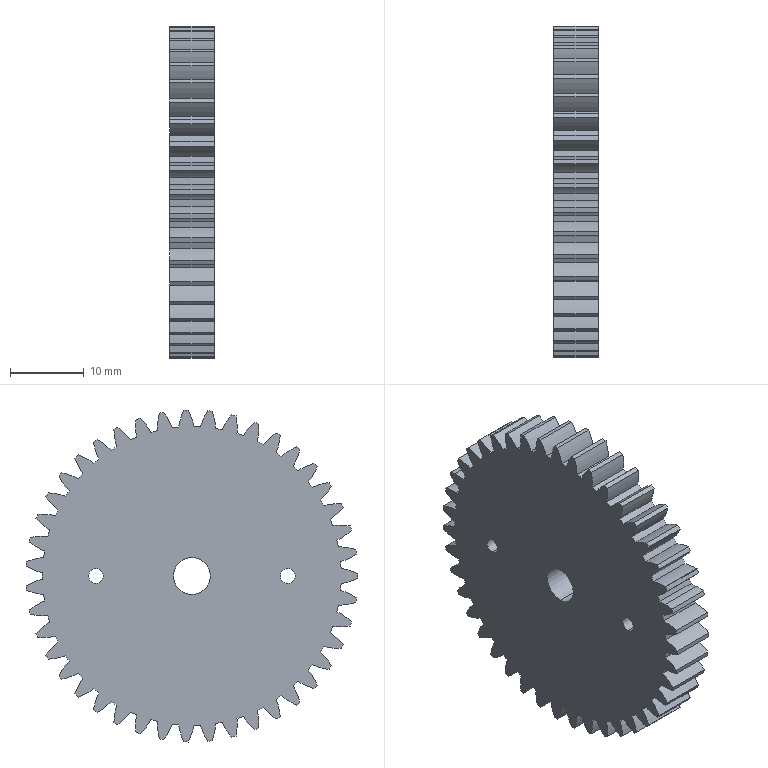Part | SolidWorks | features Boss 3, Cut 3, CirPattern 2, Fillet 2, ICE 1, Revolution 1 | 1 solid | 184 faces | box 6 x 44.961 x 44.988 mm | volume 8422 mm3 | cylinder 182 | plane 2 | commonest cylinder face diameters 17.2 x90 40.498 x43 45 x43 2 x4 5 x2